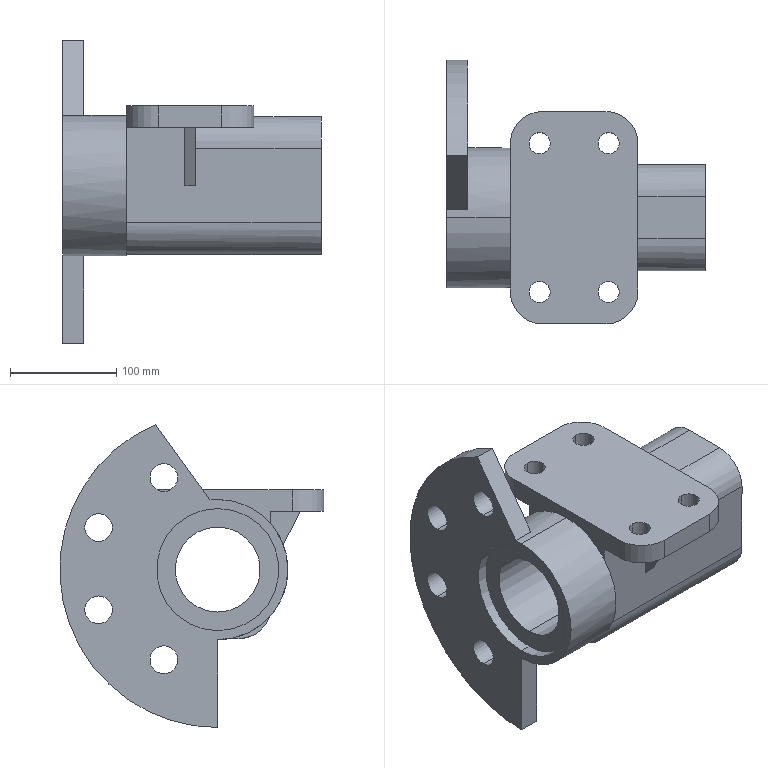Part | NX | features BREP 1 | 1 solid | 72 faces | box 243.527 x 248.694 x 285.284 mm | volume 2646572 mm3 | cylinder 38 | plane 34 | commonest cylinder face diameters 20 x8 26.115 x8 45 x8 60 x7 80 x2 115 x2